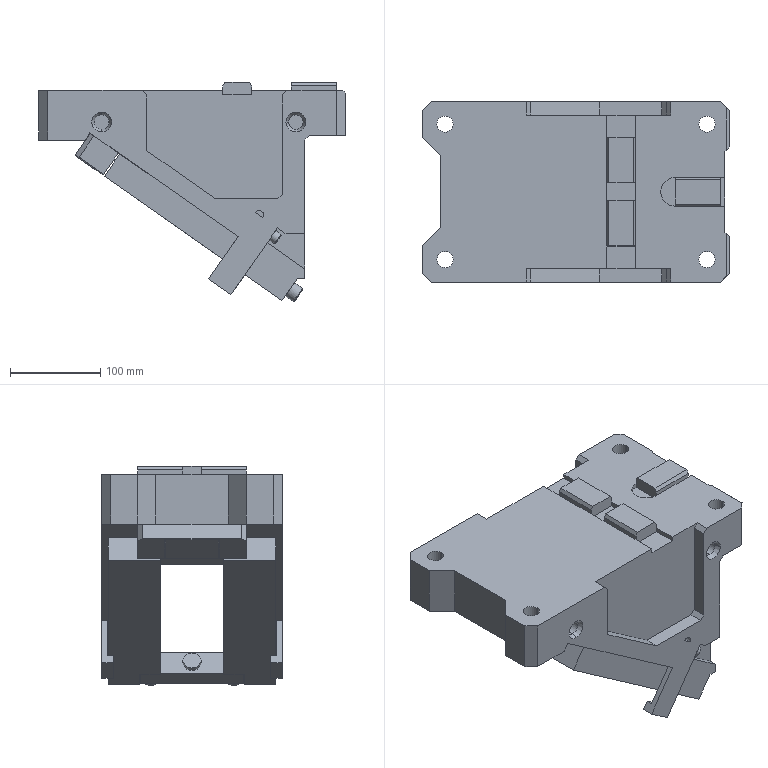Part | NX | features solid 2 | 1 solid | 219 faces | box 340 x 200 x 242.922 mm | volume 5814764 mm3 | plane 162 | cylinder 41 | cone 16 | commonest cylinder face diameters 18 x12 16 x8 26 x8 2 x4 13 x4 10 x2